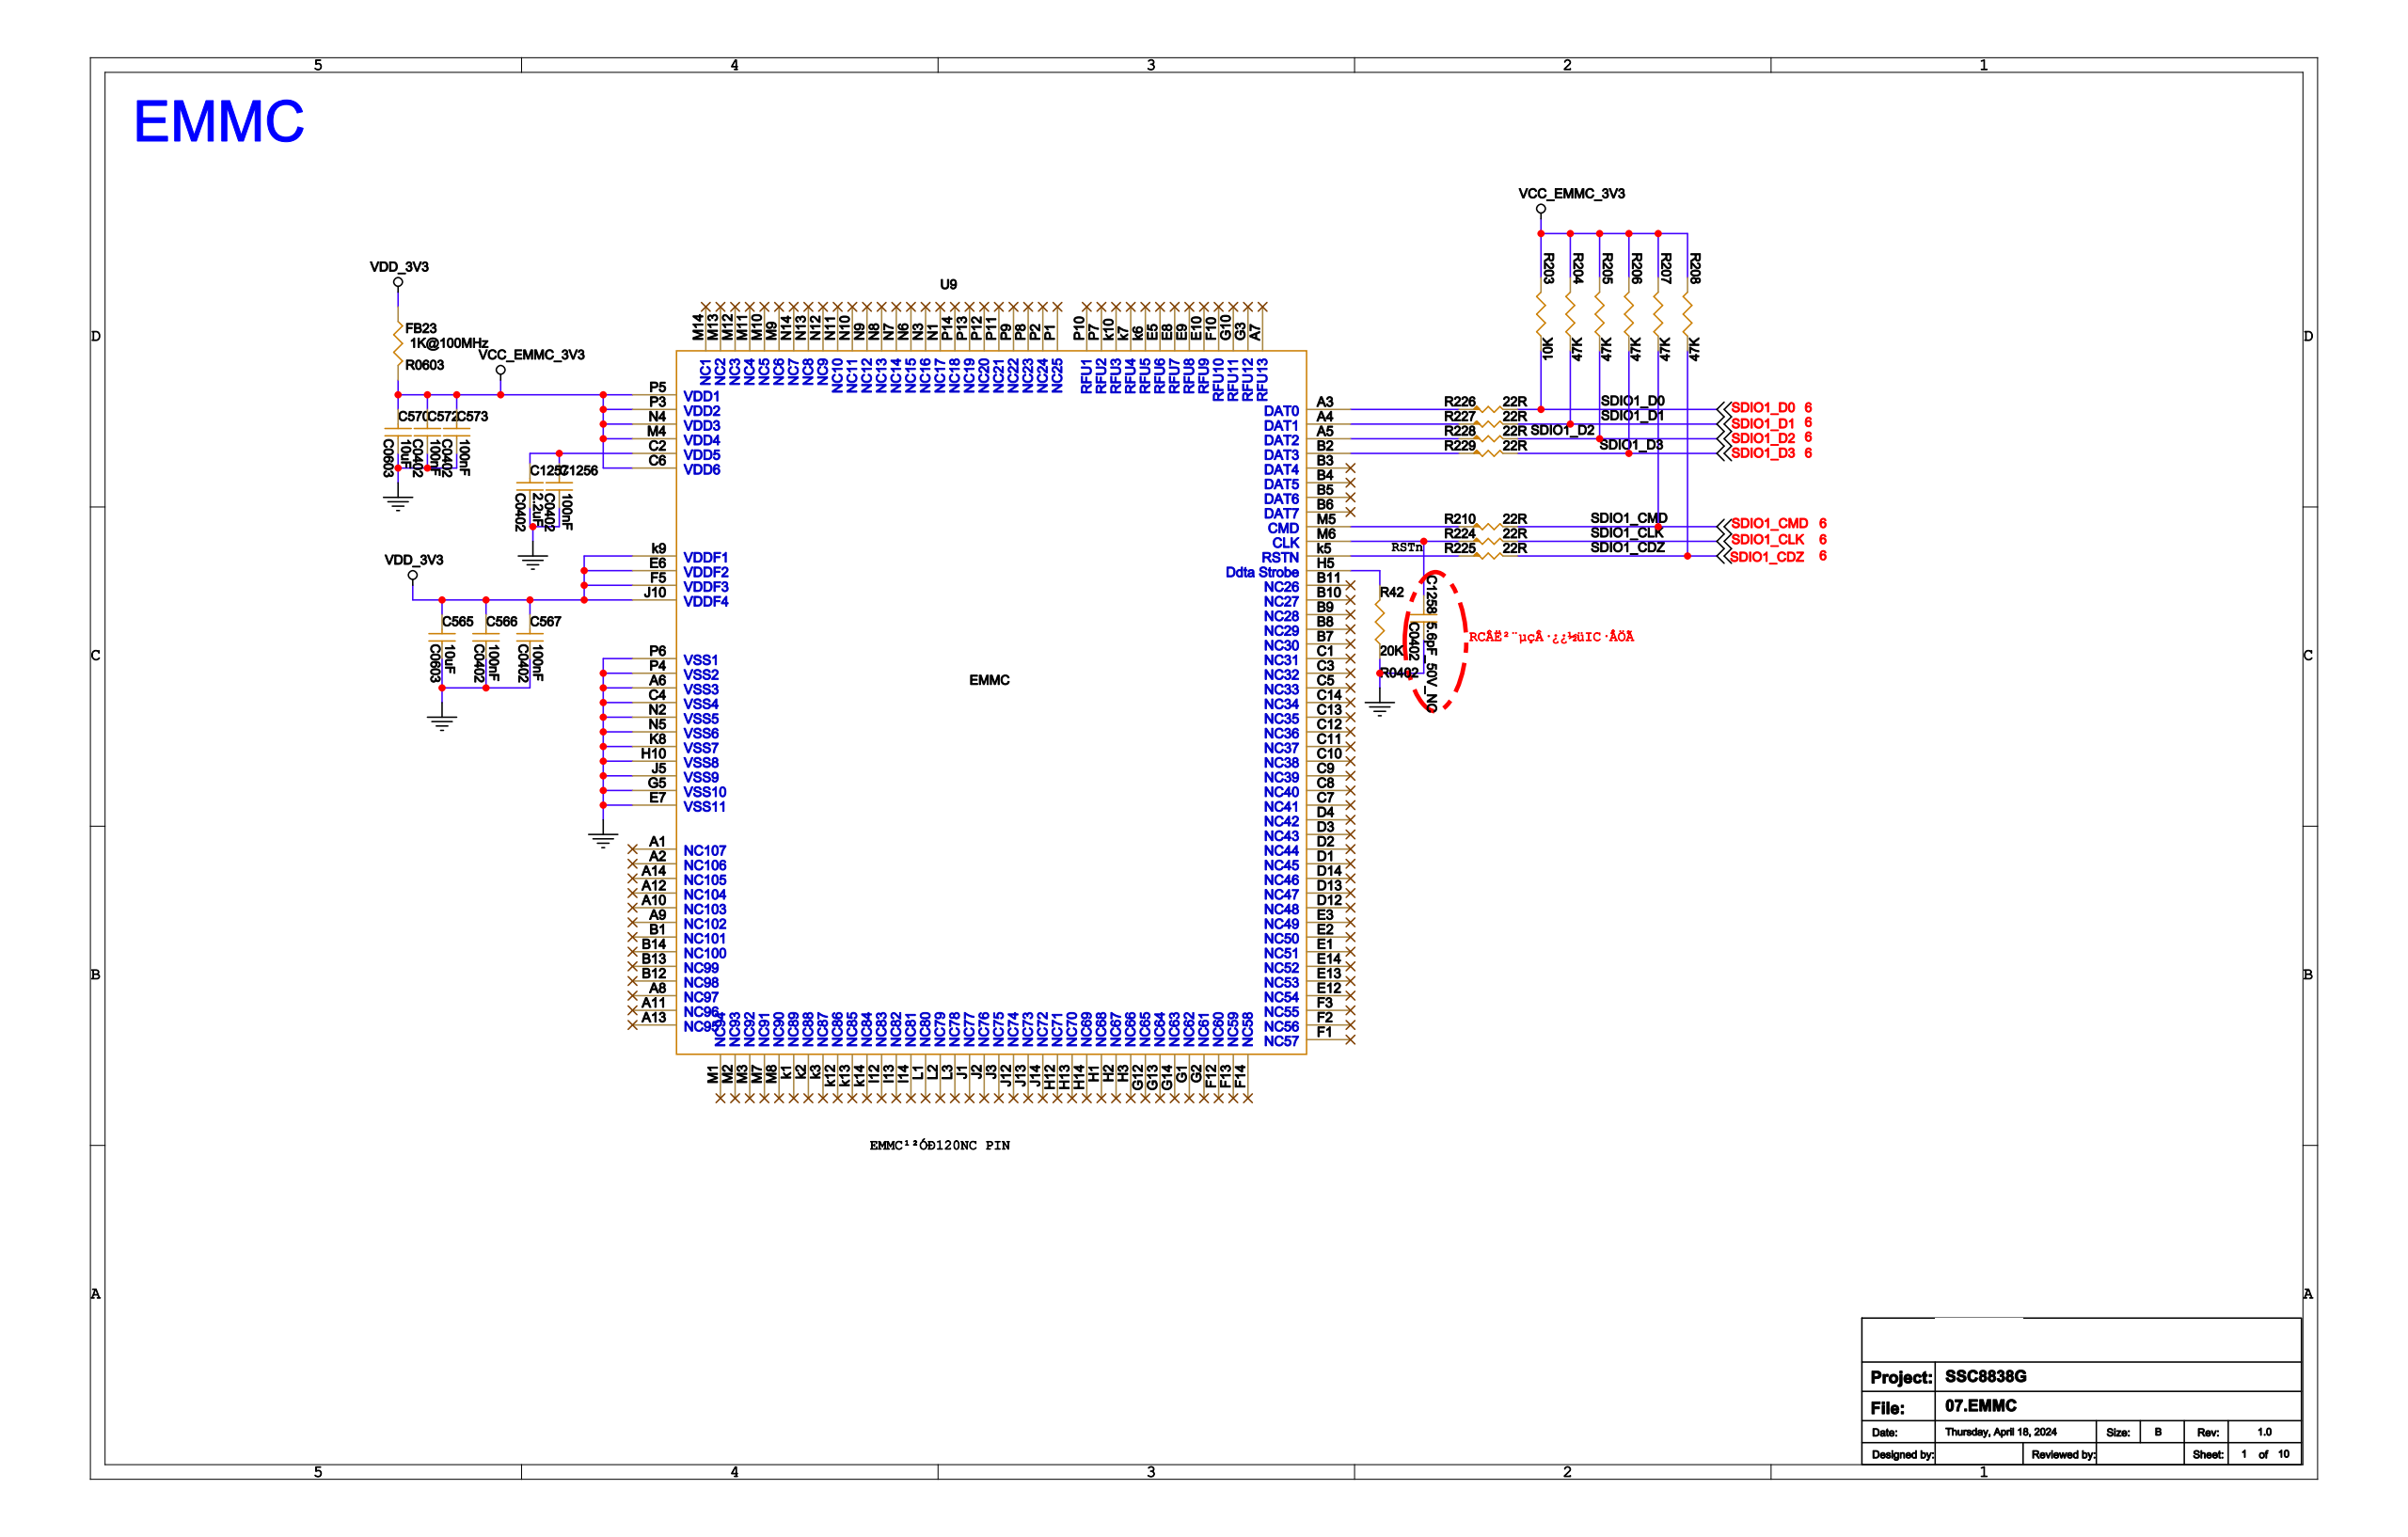Circuit board | Cadence Allegro | 958 parts | 601 nets | one sheet of the schematic
Parts on this sheet (reference | value | footprint):
C565 | 10uF | C0603
C566 | 100nF | C0402
C567 | 100nF | C0402
C570 | 10uF | C0603
C572 | 100nF | C0402
C573 | 100nF | C0402
C1256 | 100nF | C0402
C1257 | 2.2uF | C0402
C1258 | 5.6pF_50V_NC | C0402
FB23 | 1K@100MHz | R0603
R42 | 20K | R0402
R203 | 10K | R0402
R204 | 47K | R0402
R205 | 47K | R0402
R206 | 47K | R0402
R207 | 47K | R0402
R208 | 47K | R0402
R210 | 22R | R0402
R224 | 22R | R0402
R225 | 22R | R0402
R226 | 22R | R0402
R227 | 22R | R0402
R228 | 22R | R0402
R229 | 22R | R0402
U9 | EMMC | BGA153-11_5X13-P0_5-H0_8
Nets of these parts (net: part-pin ...):
GND: C565-1 C566-1 C567-1 C570-1 C572-1 C573-1 C1256-1 C1257-1 C1258-1 R42-1 U9-A6 U9-C4 U9-E7 U9-G5 U9-H10 U9-J5 U9-K8 U9-N2 U9-N5 U9-P4 U9-P6
3V3_NORMAL: C565-2 C566-2 C567-2 FB23-1 U9-E6 U9-F5 U9-J10
N22219325: C1258-2 R224-1 U9-M6
N22219534: C1256-2 C1257-2 U9-C2
VCC_EMMC_3V3: C570-2 C572-2 C573-2 FB23-2 R203-1 R204-1 R205-1 R206-1 R207-1 R208-1 U9-C6 U9-M4 U9-N4 U9-P3 U9-P5
SDIO1_D0: R203-2 R226-2
SDIO1_D1: R204-2 R227-2
SDIO1_D2: R205-2 R228-2
SDIO1_D3: R206-2 R229-2
SDIO1_CMD: R207-2 R210-2
SDIO1_CDZ: R208-2 R225-2
N22219891: R210-1 U9-M5
SDIO1_CLK: R224-2
RSTN: R225-1
N22219522: R226-1 U9-A3
N22219520: R227-1 U9-A4
N22219516: R228-1 U9-A5
N22219518: R229-1 U9-B2
N22219514: R42-2 U9-H5